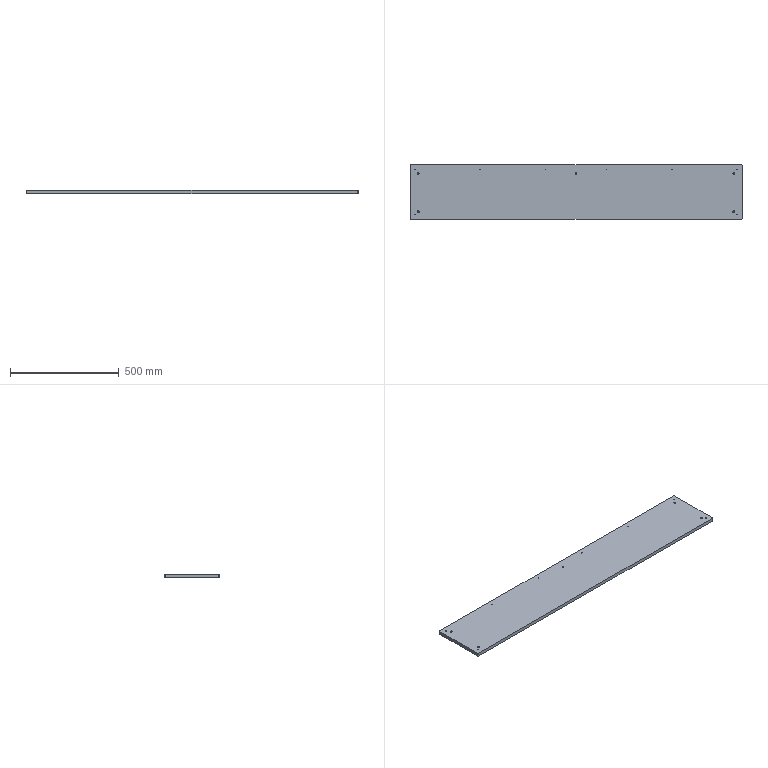Part | NX | features BREP 1 | 1 solid | 51 faces | box 1526 x 252 x 16 mm | volume 6141553 mm3 | cylinder 36 | plane 15 | commonest cylinder face diameters 3.3 x16 9 x10 15 x10